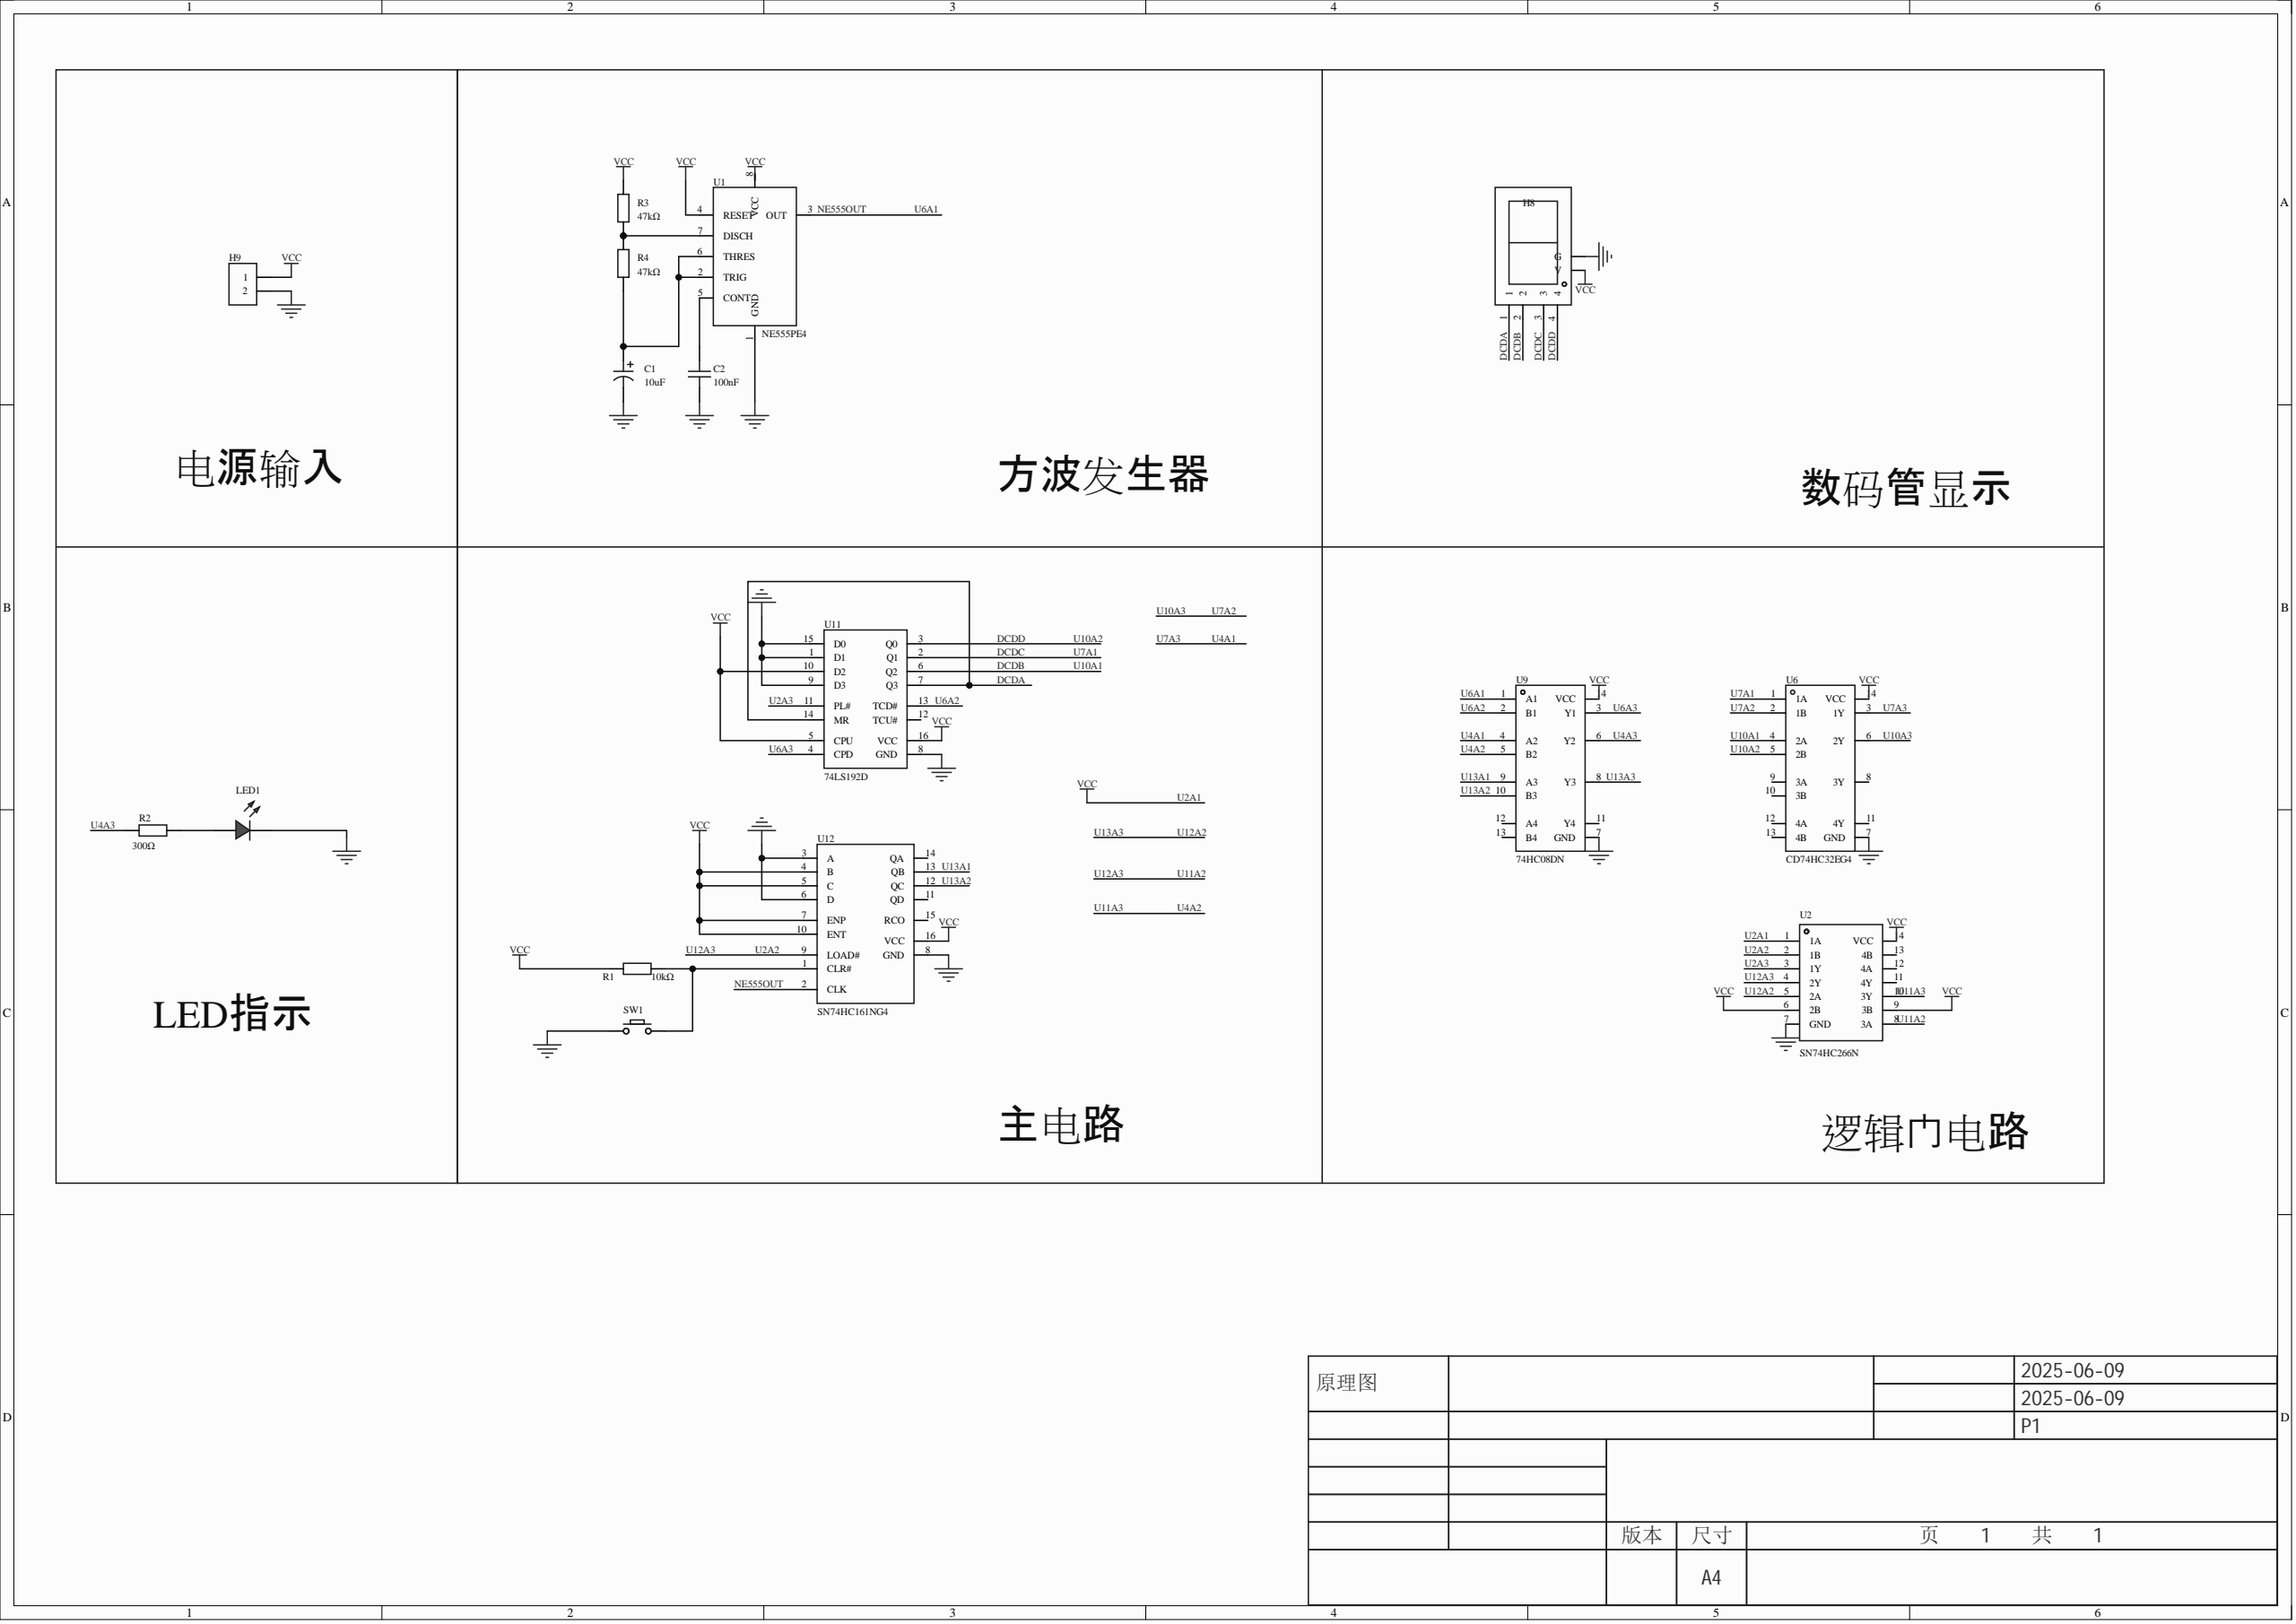Circuit board | Altium Designer | 16 parts | 23 nets
Bill of materials:
Comment,Description,Designator,Footprint,LibRef,Quantity
"10uF","容值:10uF;精度:±20%;额定电压:63V;","C1","CAP-TH_BD5.0-P2.00-D0.5-FD","SHG63V10UF03EC0822","1"
"100nF","容值:100nF;精度:±10%;额定电压:50V;温度系数:X8R;","C2","CAP-TH_L4.5-W3.0-P2.50-D0.5","FA14X8R1H104KNU00","1"
"","","H8","HDR-TH_6P-P2.54-V-M-1","HDR-M_2.54_1x6P","1"
"","","H9","HDR-TH_2P-P2.54-V-F","HDR-F_2.54_1x2P","1"
"","","LED1","LED_TH-3mm","LED_TH-R_3mm","1"
"10kΩ","","R1","Res_1/8W","Res_AXIAL-1/8W","1"
"300Ω","","R2","Res_1/8W","Res_AXIAL-1/8W","1"
"47kΩ","","R3, R4","Res_1/8W","Res_AXIAL-1/8W","2"
"","","SW1","Key_TH_3.5x6x4.3","Key_TH_3.5x6x4.3","1"
"NE555PE4","单精度计时器 8-PDIP 0 to 70","U1","PDIP-8_L9.6-W6.4-P2.54-LS7.9-BL-1","NE555PE4","1"
"SN74HC266N","逻辑类型:异或非门;通道数:4;电源电压:2V~6V;静态电流(最大值):2uA;最大传播延迟:23ns@6V,50pF;","U2","PDIP-14_L19.3-W6.4-P2.54-LS7.6-BL","SN74HC266N","1"
"CD74HC32EG4","","U6","PDIP-14_L19.3-W6.4-P2.54-LS7.6-BL","CD74HC32EG4","1"
"74HC08DN","","U9","PDIP-14_L19.3-W6.5-P2.54-LS7.6-BL","74HC08DN","1"
"74LS192D","工作电压:2V~6V;元件数:1;触发沿:上升沿;计数速率:24MHz;","U11","PDIP-16_L19.3-W6.4-P2.54-LS7.94-BL","SN74LS192N(LX)","1"
"SN74HC161NG4","工作电压:2V~6V;元件数:1;触发沿:上升沿;计数速率:36MHz;","U12","PDIP-16_L19.3-W6.4-P2.54-LS7.9-BL","SN74HC161NG4","1"
Netlist (Protel format):
[
C1
CAP-TH_BD5.0-P2.00-D0.5-FD
10uF



]
[
C2
CAP-TH_L4.5-W3.0-P2.50-D0.5
100nF



]
[
H8
HDR-TH_6P-P2.54-V-M-1




]
[
H9
HDR-TH_2P-P2.54-V-F




]
[
LED1
LED_TH-3mm




]
[
R1
Res_1/8W
10kΩ



]
[
R2
Res_1/8W
300Ω



]
[
R3
Res_1/8W
47kΩ



]
[
R4
Res_1/8W
47kΩ



]
[
SW1
Key_TH_3.5x6x4.3




]
[
U1
PDIP-8_L9.6-W6.4-P2.54-LS7.9-BL-1
NE555PE4



]
[
U2
PDIP-14_L19.3-W6.4-P2.54-LS7.6-BL
SN74HC266N



]
[
U6
PDIP-14_L19.3-W6.4-P2.54-LS7.6-BL
CD74HC32EG4



]
[
U9
PDIP-14_L19.3-W6.5-P2.54-LS7.6-BL
74HC08DN



]
[
U11
PDIP-16_L19.3-W6.4-P2.54-LS7.94-BL
74LS192D



]
[
U12
PDIP-16_L19.3-W6.4-P2.54-LS7.9-BL
SN74HC161NG4



]
(
U13A2
U9-10
U12-12
)
(
U13A1
U9-9
U12-13
)
(
U12A2
U2-5
U9-8
)
(
U7A2
U6-2
U6-6
)
(
U6A3
U9-3
U11-4
)
(
U6A2
U9-2
U11-13
)
(
U4A3
R2-2
U9-6
)
(
U4A2
U2-10
U9-5
)
(
U4A1
U6-3
U9-4
)
(
U2A3
U2-3
U11-11
)
(
U2A2
U2-2
U2-4
U2-8
U12-9
)
(
U2A1
H8-5
H9-1
R1-1
R3-2
U1-4
U1-8
U2-1
U2-6
U2-9
U2-14
U6-14
U9-14
U11-5
U11-10
U11-16
U12-4
U12-5
U12-7
U12-10
U12-16
)
(
NetR3_1
R3-1
R4-2
U1-7
)
(
NetR1_2
R1-2
SW1-B
U12-1
)
(
NetLED1_1
LED1-1
R2-1
)
(
NetC2_2
C2-2
U1-5
)
(
NetC1_1
C1-1
R4-1
U1-2
U1-6
)
(
NE555OUT
U1-3
U9-1
U12-2
)
(
GND
C1-2
C2-1
H8-6
H9-2
LED1-2
SW1-A
U1-1
U2-7
U6-7
U9-7
U11-1
U11-8
U11-9
U11-15
U12-3
U12-6
U12-8
)
(
DCDD
H8-4
U6-5
U11-3
)
(
DCDC
H8-3
U6-1
U11-2
)
(
DCDB
H8-2
U6-4
U11-6
)
(
DCDA
H8-1
U11-7
U11-14
)